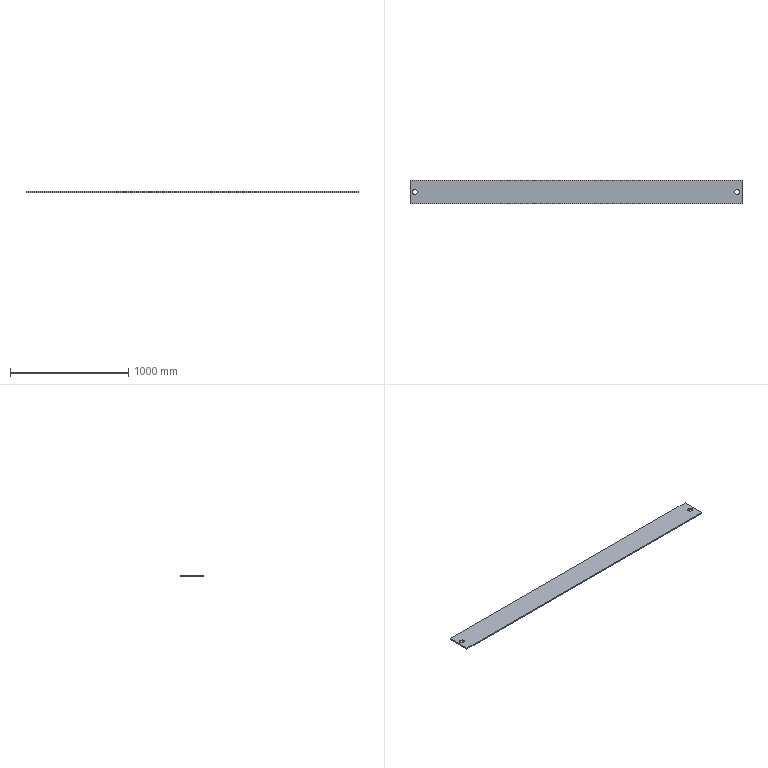Part | NX | features BREP 1 | 1 solid | 10 faces | box 2807 x 200 x 10 mm | volume 5588867 mm3 | plane 6 | cylinder 4 | commonest cylinder face diameters 40 x4
STEP:
#1=CARTESIAN_POINT('',(1343.5,0.,-5.));
#2=VERTEX_POINT('',#1);
#3=CARTESIAN_POINT('',(1383.5,0.,-5.));
#4=VERTEX_POINT('',#3);
#5=CARTESIAN_POINT('',(1363.5,0.,-5.));
#6=DIRECTION('',(0.,0.,1.));
#7=DIRECTION('',(-1.,0.,0.));
#8=AXIS2_PLACEMENT_3D('',#5,#6,#7);
#9=CIRCLE('',#8,20.);
#10=EDGE_CURVE('',#2,#4,#9,.T.);
#11=ORIENTED_EDGE('',*,*,#10,.F.);
#12=CARTESIAN_POINT('',(1343.5,0.,5.));
#13=VERTEX_POINT('',#12);
#14=CARTESIAN_POINT('',(1343.5,0.,-5.));
#15=DIRECTION('',(0.,0.,1.));
#16=VECTOR('',#15,1000.);
#17=LINE('',#14,#16);
#18=EDGE_CURVE('',#2,#13,#17,.T.);
#19=ORIENTED_EDGE('',*,*,#18,.T.);
#20=CARTESIAN_POINT('',(1383.5,0.,5.));
#21=VERTEX_POINT('',#20);
#22=CARTESIAN_POINT('',(1363.5,0.,5.));
#23=DIRECTION('',(0.,0.,1.));
#24=DIRECTION('',(-1.,0.,0.));
#25=AXIS2_PLACEMENT_3D('',#22,#23,#24);
#26=CIRCLE('',#25,20.);
#27=EDGE_CURVE('',#13,#21,#26,.T.);
#28=ORIENTED_EDGE('',*,*,#27,.T.);
#29=CARTESIAN_POINT('',(1383.5,0.,-5.));
#30=DIRECTION('',(0.,0.,1.));
#31=VECTOR('',#30,1000.);
#32=LINE('',#29,#31);
#33=EDGE_CURVE('',#4,#21,#32,.T.);
#34=ORIENTED_EDGE('',*,*,#33,.F.);
#35=EDGE_LOOP('',(#11,#19,#28,#34));
#36=FACE_BOUND('',#35,.T.);
#37=CARTESIAN_POINT('',(1363.5,0.,-5.));
#38=DIRECTION('',(0.,0.,1.));
#39=DIRECTION('',(-1.,0.,0.));
#40=AXIS2_PLACEMENT_3D('',#37,#38,#39);
#41=CYLINDRICAL_SURFACE('',#40,20.);
#42=ADVANCED_FACE('',(#36),#41,.F.);
#43=CARTESIAN_POINT('',(-1383.5,0.,-5.));
#44=VERTEX_POINT('',#43);
#45=CARTESIAN_POINT('',(-1343.5,0.,-5.));
#46=VERTEX_POINT('',#45);
#47=CARTESIAN_POINT('',(-1363.5,0.,-5.));
#48=DIRECTION('',(0.,0.,1.));
#49=DIRECTION('',(1.,0.,0.));
#50=AXIS2_PLACEMENT_3D('',#47,#48,#49);
#51=CIRCLE('',#50,20.);
#52=EDGE_CURVE('',#44,#46,#51,.T.);
#53=ORIENTED_EDGE('',*,*,#52,.F.);
#54=CARTESIAN_POINT('',(-1383.5,0.,5.));
#55=VERTEX_POINT('',#54);
#56=CARTESIAN_POINT('',(-1383.5,0.,-5.));
#57=DIRECTION('',(0.,0.,1.));
#58=VECTOR('',#57,1000.);
#59=LINE('',#56,#58);
#60=EDGE_CURVE('',#44,#55,#59,.T.);
#61=ORIENTED_EDGE('',*,*,#60,.T.);
#62=CARTESIAN_POINT('',(-1343.5,0.,5.));
#63=VERTEX_POINT('',#62);
#64=CARTESIAN_POINT('',(-1363.5,0.,5.));
#65=DIRECTION('',(0.,0.,1.));
#66=DIRECTION('',(1.,0.,0.));
#67=AXIS2_PLACEMENT_3D('',#64,#65,#66);
#68=CIRCLE('',#67,20.);
#69=EDGE_CURVE('',#55,#63,#68,.T.);
#70=ORIENTED_EDGE('',*,*,#69,.T.);
#71=CARTESIAN_POINT('',(-1343.5,0.,-5.));
#72=DIRECTION('',(0.,0.,1.));
#73=VECTOR('',#72,1000.);
#74=LINE('',#71,#73);
#75=EDGE_CURVE('',#46,#63,#74,.T.);
#76=ORIENTED_EDGE('',*,*,#75,.F.);
#77=EDGE_LOOP('',(#53,#61,#70,#76));
#78=FACE_BOUND('',#77,.T.);
#79=CARTESIAN_POINT('',(-1363.5,0.,-5.));
#80=DIRECTION('',(0.,0.,1.));
#81=DIRECTION('',(-1.,0.,0.));
#82=AXIS2_PLACEMENT_3D('',#79,#80,#81);
#83=CYLINDRICAL_SURFACE('',#82,20.);
#84=ADVANCED_FACE('',(#78),#83,.F.);
#85=CARTESIAN_POINT('',(-1403.5,100.,-5.));
#86=VERTEX_POINT('',#85);
#87=CARTESIAN_POINT('',(-1403.5,-100.,-5.));
#88=VERTEX_POINT('',#87);
#89=CARTESIAN_POINT('',(-1403.5,100.,-5.));
#90=DIRECTION('',(0.,-1.,0.));
#91=VECTOR('',#90,1000.);
#92=LINE('',#89,#91);
#93=EDGE_CURVE('',#86,#88,#92,.T.);
#94=ORIENTED_EDGE('',*,*,#93,.T.);
#95=CARTESIAN_POINT('',(-1403.5,-100.,5.));
#96=VERTEX_POINT('',#95);
#97=CARTESIAN_POINT('',(-1403.5,-100.,5.));
#98=DIRECTION('',(0.,0.,-1.));
#99=VECTOR('',#98,1000.);
#100=LINE('',#97,#99);
#101=EDGE_CURVE('',#96,#88,#100,.T.);
#102=ORIENTED_EDGE('',*,*,#101,.F.);
#103=CARTESIAN_POINT('',(-1403.5,100.,5.));
#104=VERTEX_POINT('',#103);
#105=CARTESIAN_POINT('',(-1403.5,100.,5.));
#106=DIRECTION('',(0.,-1.,0.));
#107=VECTOR('',#106,1000.);
#108=LINE('',#105,#107);
#109=EDGE_CURVE('',#104,#96,#108,.T.);
#110=ORIENTED_EDGE('',*,*,#109,.F.);
#111=CARTESIAN_POINT('',(-1403.5,100.,5.));
#112=DIRECTION('',(0.,0.,-1.));
#113=VECTOR('',#112,1000.);
#114=LINE('',#111,#113);
#115=EDGE_CURVE('',#104,#86,#114,.T.);
#116=ORIENTED_EDGE('',*,*,#115,.T.);
#117=EDGE_LOOP('',(#94,#102,#110,#116));
#118=FACE_BOUND('',#117,.T.);
#119=CARTESIAN_POINT('',(-1403.5,100.,5.));
#120=DIRECTION('',(1.,0.,0.));
#121=DIRECTION('',(0.,0.,1.));
#122=AXIS2_PLACEMENT_3D('',#119,#120,#121);
#123=PLANE('',#122);
#124=ADVANCED_FACE('',(#118),#123,.F.);
#125=CARTESIAN_POINT('',(1403.5,-100.,-5.));
#126=VERTEX_POINT('',#125);
#127=CARTESIAN_POINT('',(-1403.5,-100.,-5.));
#128=DIRECTION('',(1.,0.,0.));
#129=VECTOR('',#128,1000.);
#130=LINE('',#127,#129);
#131=EDGE_CURVE('',#88,#126,#130,.T.);
#132=ORIENTED_EDGE('',*,*,#131,.T.);
#133=CARTESIAN_POINT('',(1403.5,-100.,5.));
#134=VERTEX_POINT('',#133);
#135=CARTESIAN_POINT('',(1403.5,-100.,5.));
#136=DIRECTION('',(0.,0.,-1.));
#137=VECTOR('',#136,1000.);
#138=LINE('',#135,#137);
#139=EDGE_CURVE('',#134,#126,#138,.T.);
#140=ORIENTED_EDGE('',*,*,#139,.F.);
#141=CARTESIAN_POINT('',(-1403.5,-100.,5.));
#142=DIRECTION('',(1.,0.,0.));
#143=VECTOR('',#142,1000.);
#144=LINE('',#141,#143);
#145=EDGE_CURVE('',#96,#134,#144,.T.);
#146=ORIENTED_EDGE('',*,*,#145,.F.);
#147=ORIENTED_EDGE('',*,*,#101,.T.);
#148=EDGE_LOOP('',(#132,#140,#146,#147));
#149=FACE_BOUND('',#148,.T.);
#150=CARTESIAN_POINT('',(-1403.5,-100.,5.));
#151=DIRECTION('',(0.,1.,0.));
#152=DIRECTION('',(0.,0.,-1.));
#153=AXIS2_PLACEMENT_3D('',#150,#151,#152);
#154=PLANE('',#153);
#155=ADVANCED_FACE('',(#149),#154,.F.);
#156=CARTESIAN_POINT('',(1403.5,100.,-5.));
#157=VERTEX_POINT('',#156);
#158=CARTESIAN_POINT('',(1403.5,100.,-5.));
#159=DIRECTION('',(0.,1.,0.));
#160=VECTOR('',#159,1000.);
#161=LINE('',#158,#160);
#162=EDGE_CURVE('',#126,#157,#161,.T.);
#163=ORIENTED_EDGE('',*,*,#162,.T.);
#164=CARTESIAN_POINT('',(1403.5,100.,5.));
#165=VERTEX_POINT('',#164);
#166=CARTESIAN_POINT('',(1403.5,100.,5.));
#167=DIRECTION('',(0.,0.,-1.));
#168=VECTOR('',#167,1000.);
#169=LINE('',#166,#168);
#170=EDGE_CURVE('',#165,#157,#169,.T.);
#171=ORIENTED_EDGE('',*,*,#170,.F.);
#172=CARTESIAN_POINT('',(1403.5,100.,5.));
#173=DIRECTION('',(0.,1.,0.));
#174=VECTOR('',#173,1000.);
#175=LINE('',#172,#174);
#176=EDGE_CURVE('',#134,#165,#175,.T.);
#177=ORIENTED_EDGE('',*,*,#176,.F.);
#178=ORIENTED_EDGE('',*,*,#139,.T.);
#179=EDGE_LOOP('',(#163,#171,#177,#178));
#180=FACE_BOUND('',#179,.T.);
#181=CARTESIAN_POINT('',(1403.5,100.,5.));
#182=DIRECTION('',(-1.,0.,0.));
#183=DIRECTION('',(0.,0.,-1.));
#184=AXIS2_PLACEMENT_3D('',#181,#182,#183);
#185=PLANE('',#184);
#186=ADVANCED_FACE('',(#180),#185,.F.);
#187=CARTESIAN_POINT('',(-1403.5,100.,-5.));
#188=DIRECTION('',(-1.,0.,0.));
#189=VECTOR('',#188,1000.);
#190=LINE('',#187,#189);
#191=EDGE_CURVE('',#157,#86,#190,.T.);
#192=ORIENTED_EDGE('',*,*,#191,.T.);
#193=ORIENTED_EDGE('',*,*,#115,.F.);
#194=CARTESIAN_POINT('',(-1403.5,100.,5.));
#195=DIRECTION('',(-1.,0.,0.));
#196=VECTOR('',#195,1000.);
#197=LINE('',#194,#196);
#198=EDGE_CURVE('',#165,#104,#197,.T.);
#199=ORIENTED_EDGE('',*,*,#198,.F.);
#200=ORIENTED_EDGE('',*,*,#170,.T.);
#201=EDGE_LOOP('',(#192,#193,#199,#200));
#202=FACE_BOUND('',#201,.T.);
#203=CARTESIAN_POINT('',(-1403.5,100.,5.));
#204=DIRECTION('',(0.,-1.,0.));
#205=DIRECTION('',(0.,0.,1.));
#206=AXIS2_PLACEMENT_3D('',#203,#204,#205);
#207=PLANE('',#206);
#208=ADVANCED_FACE('',(#202),#207,.F.);
#209=CARTESIAN_POINT('',(1363.5,0.,5.));
#210=DIRECTION('',(0.,0.,1.));
#211=DIRECTION('',(-1.,0.,0.));
#212=AXIS2_PLACEMENT_3D('',#209,#210,#211);
#213=CIRCLE('',#212,20.);
#214=EDGE_CURVE('',#21,#13,#213,.T.);
#215=ORIENTED_EDGE('',*,*,#214,.F.);
#216=ORIENTED_EDGE('',*,*,#27,.F.);
#217=EDGE_LOOP('',(#215,#216));
#218=FACE_BOUND('',#217,.T.);
#219=CARTESIAN_POINT('',(-1363.5,0.,5.));
#220=DIRECTION('',(0.,0.,1.));
#221=DIRECTION('',(1.,0.,0.));
#222=AXIS2_PLACEMENT_3D('',#219,#220,#221);
#223=CIRCLE('',#222,20.);
#224=EDGE_CURVE('',#63,#55,#223,.T.);
#225=ORIENTED_EDGE('',*,*,#224,.F.);
#226=ORIENTED_EDGE('',*,*,#69,.F.);
#227=EDGE_LOOP('',(#225,#226));
#228=FACE_BOUND('',#227,.T.);
#229=ORIENTED_EDGE('',*,*,#109,.T.);
#230=ORIENTED_EDGE('',*,*,#145,.T.);
#231=ORIENTED_EDGE('',*,*,#176,.T.);
#232=ORIENTED_EDGE('',*,*,#198,.T.);
#233=EDGE_LOOP('',(#229,#230,#231,#232));
#234=FACE_BOUND('',#233,.T.);
#235=CARTESIAN_POINT('',(-1403.5,-100.,5.));
#236=DIRECTION('',(0.,0.,1.));
#237=DIRECTION('',(-1.,0.,0.));
#238=AXIS2_PLACEMENT_3D('',#235,#236,#237);
#239=PLANE('',#238);
#240=ADVANCED_FACE('',(#218,#228,#234),#239,.T.);
#241=CARTESIAN_POINT('',(1363.5,0.,-5.));
#242=DIRECTION('',(0.,0.,1.));
#243=DIRECTION('',(-1.,0.,0.));
#244=AXIS2_PLACEMENT_3D('',#241,#242,#243);
#245=CIRCLE('',#244,20.);
#246=EDGE_CURVE('',#4,#2,#245,.T.);
#247=ORIENTED_EDGE('',*,*,#246,.T.);
#248=ORIENTED_EDGE('',*,*,#10,.T.);
#249=EDGE_LOOP('',(#247,#248));
#250=FACE_BOUND('',#249,.T.);
#251=CARTESIAN_POINT('',(-1363.5,0.,-5.));
#252=DIRECTION('',(0.,0.,1.));
#253=DIRECTION('',(1.,0.,0.));
#254=AXIS2_PLACEMENT_3D('',#251,#252,#253);
#255=CIRCLE('',#254,20.);
#256=EDGE_CURVE('',#46,#44,#255,.T.);
#257=ORIENTED_EDGE('',*,*,#256,.T.);
#258=ORIENTED_EDGE('',*,*,#52,.T.);
#259=EDGE_LOOP('',(#257,#258));
#260=FACE_BOUND('',#259,.T.);
#261=ORIENTED_EDGE('',*,*,#93,.F.);
#262=ORIENTED_EDGE('',*,*,#191,.F.);
#263=ORIENTED_EDGE('',*,*,#162,.F.);
#264=ORIENTED_EDGE('',*,*,#131,.F.);
#265=EDGE_LOOP('',(#261,#262,#263,#264));
#266=FACE_BOUND('',#265,.T.);
#267=CARTESIAN_POINT('',(-1403.5,-100.,-5.));
#268=DIRECTION('',(0.,0.,1.));
#269=DIRECTION('',(-1.,0.,0.));
#270=AXIS2_PLACEMENT_3D('',#267,#268,#269);
#271=PLANE('',#270);
#272=ADVANCED_FACE('',(#250,#260,#266),#271,.F.);
#273=ORIENTED_EDGE('',*,*,#60,.F.);
#274=ORIENTED_EDGE('',*,*,#256,.F.);
#275=ORIENTED_EDGE('',*,*,#75,.T.);
#276=ORIENTED_EDGE('',*,*,#224,.T.);
#277=EDGE_LOOP('',(#273,#274,#275,#276));
#278=FACE_BOUND('',#277,.T.);
#279=CARTESIAN_POINT('',(-1363.5,0.,-5.));
#280=DIRECTION('',(0.,0.,1.));
#281=DIRECTION('',(-1.,0.,0.));
#282=AXIS2_PLACEMENT_3D('',#279,#280,#281);
#283=CYLINDRICAL_SURFACE('',#282,20.);
#284=ADVANCED_FACE('',(#278),#283,.F.);
#285=ORIENTED_EDGE('',*,*,#18,.F.);
#286=ORIENTED_EDGE('',*,*,#246,.F.);
#287=ORIENTED_EDGE('',*,*,#33,.T.);
#288=ORIENTED_EDGE('',*,*,#214,.T.);
#289=EDGE_LOOP('',(#285,#286,#287,#288));
#290=FACE_BOUND('',#289,.T.);
#291=CARTESIAN_POINT('',(1363.5,0.,-5.));
#292=DIRECTION('',(0.,0.,1.));
#293=DIRECTION('',(-1.,0.,0.));
#294=AXIS2_PLACEMENT_3D('',#291,#292,#293);
#295=CYLINDRICAL_SURFACE('',#294,20.);
#296=ADVANCED_FACE('',(#290),#295,.F.);
#297=CLOSED_SHELL('',(#42,#84,#124,#155,#186,#208,#240,#272,#284,#296));
#298=MANIFOLD_SOLID_BREP('',#297);
#299=(LENGTH_UNIT()NAMED_UNIT(*)SI_UNIT(.MILLI.,.METRE.));
#300=UNCERTAINTY_MEASURE_WITH_UNIT(LENGTH_MEASURE(0.00001),#299,'','');
#301=(NAMED_UNIT(*)PLANE_ANGLE_UNIT()SI_UNIT($,.RADIAN.));
#302=(NAMED_UNIT(*)SI_UNIT($,.STERADIAN.)SOLID_ANGLE_UNIT());
#303=(GEOMETRIC_REPRESENTATION_CONTEXT(3)GLOBAL_UNCERTAINTY_ASSIGNED_CONTEXT((#300))GLOBAL_UNIT_ASSIGNED_CONTEXT((#299,#301,#302))REPRESENTATION_CONTEXT('',''));
#304=ADVANCED_BREP_SHAPE_REPRESENTATION('',(#298),#303);